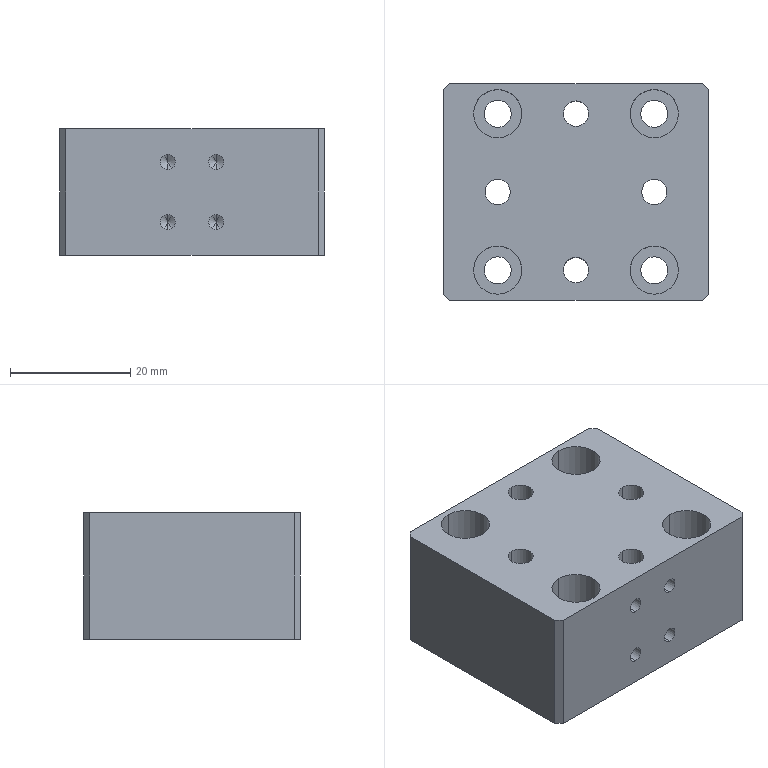NC program | NX | posted with a generic post | part box 44 x 36 x 21 mm
Whole program:
N10 G17 G21 G94 G90
(DRILLING_COPY_1_COPY , TOOL : D6A45)
N12 T07 M6
N14 G54
N16 G17 G0 G90 X-4. Y-5. B0. C0. S5000 M3
N18 G43 Z30. H7
N20 G94 G81 G98 Z-1.6 F250. R3.
N22 X4. Y5.
N24 Y-5.
N26 X-4. Y5.
N28 G80
N30 G0 X-4. Y5. Z30.
N32 M5
(DRILLING_COPY_COPY_2 , TOOL : 2.5ZT)
N34 T12 M6
N36 G54
N38 G17 G0 G90 X-4. Y-5. B0. C0. S2000 M3
N40 G43 Z30. H12
N42 G94 G83 G98 Z-8.251 F150. Q2. R3.
N44 X4. Y5.
N46 Y-5.
N48 X-4. Y5.
N50 G80
N52 G0 X-4. Y5. Z30.
N54 M5
N56 M2